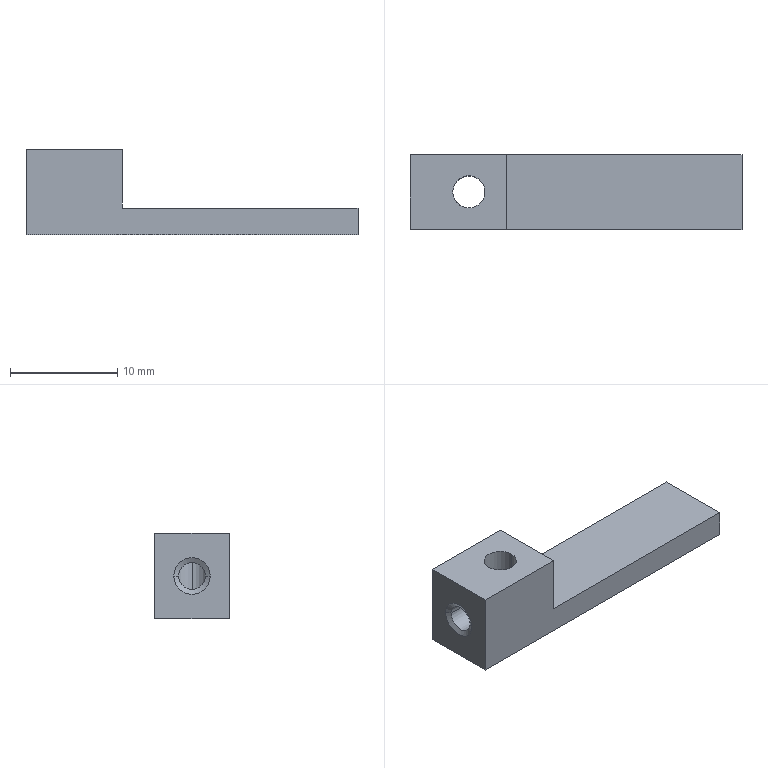Part | NX | 1 solid | 14 faces | box 31 x 7 x 8 mm | volume 811.579 mm3 | plane 8 | cylinder 4 | cone 2 | commonest cylinder face diameters 2.5 x2 3 x2
STEP:
#1=CARTESIAN_POINT('',(-15.5,3.5,-4.));
#2=VERTEX_POINT('',#1);
#3=CARTESIAN_POINT('',(-15.5,-3.5,-4.));
#4=VERTEX_POINT('',#3);
#5=CARTESIAN_POINT('',(-15.5,0.,-4.));
#6=DIRECTION('',(0.,-1.,0.));
#7=VECTOR('',#6,1000.);
#8=LINE('',#5,#7);
#9=EDGE_CURVE('',#2,#4,#8,.T.);
#10=ORIENTED_EDGE('',*,*,#9,.F.);
#11=CARTESIAN_POINT('',(15.5,3.5,-4.));
#12=VERTEX_POINT('',#11);
#13=CARTESIAN_POINT('',(-15.5,3.5,-4.));
#14=DIRECTION('',(1.,0.,0.));
#15=VECTOR('',#14,1000.);
#16=LINE('',#13,#15);
#17=EDGE_CURVE('',#2,#12,#16,.T.);
#18=ORIENTED_EDGE('',*,*,#17,.T.);
#19=CARTESIAN_POINT('',(15.5,-3.5,-4.));
#20=VERTEX_POINT('',#19);
#21=CARTESIAN_POINT('',(15.5,3.5,-4.));
#22=DIRECTION('',(0.,-1.,0.));
#23=VECTOR('',#22,1000.);
#24=LINE('',#21,#23);
#25=EDGE_CURVE('',#12,#20,#24,.T.);
#26=ORIENTED_EDGE('',*,*,#25,.T.);
#27=CARTESIAN_POINT('',(15.5,-3.5,-4.));
#28=DIRECTION('',(-1.,0.,0.));
#29=VECTOR('',#28,1000.);
#30=LINE('',#27,#29);
#31=EDGE_CURVE('',#20,#4,#30,.T.);
#32=ORIENTED_EDGE('',*,*,#31,.T.);
#33=EDGE_LOOP('',(#10,#18,#26,#32));
#34=FACE_BOUND('',#33,.T.);
#35=CARTESIAN_POINT('',(-8.5,0.,-4.));
#36=VERTEX_POINT('',#35);
#37=CARTESIAN_POINT('',(-11.5,0.,-4.));
#38=VERTEX_POINT('',#37);
#39=CARTESIAN_POINT('',(-10.,0.,-4.));
#40=DIRECTION('',(0.,0.,1.));
#41=DIRECTION('',(1.,0.,0.));
#42=AXIS2_PLACEMENT_3D('',#39,#40,#41);
#43=CIRCLE('',#42,1.5);
#44=EDGE_CURVE('',#36,#38,#43,.T.);
#45=ORIENTED_EDGE('',*,*,#44,.T.);
#46=CARTESIAN_POINT('',(-10.,0.,-4.));
#47=DIRECTION('',(0.,0.,1.));
#48=DIRECTION('',(1.,0.,0.));
#49=AXIS2_PLACEMENT_3D('',#46,#47,#48);
#50=CIRCLE('',#49,1.5);
#51=EDGE_CURVE('',#38,#36,#50,.T.);
#52=ORIENTED_EDGE('',*,*,#51,.T.);
#53=EDGE_LOOP('',(#45,#52));
#54=FACE_BOUND('',#53,.T.);
#55=CARTESIAN_POINT('',(0.,0.,-4.));
#56=DIRECTION('',(0.,0.,1.));
#57=DIRECTION('',(1.,0.,0.));
#58=AXIS2_PLACEMENT_3D('',#55,#56,#57);
#59=PLANE('',#58);
#60=ADVANCED_FACE('',(#34,#54),#59,.F.);
#61=ORIENTED_EDGE('',*,*,#9,.T.);
#62=CARTESIAN_POINT('',(-15.5,-3.5,4.));
#63=VERTEX_POINT('',#62);
#64=CARTESIAN_POINT('',(-15.5,-3.5,0.));
#65=DIRECTION('',(0.,0.,-1.));
#66=VECTOR('',#65,1000.);
#67=LINE('',#64,#66);
#68=EDGE_CURVE('',#63,#4,#67,.T.);
#69=ORIENTED_EDGE('',*,*,#68,.F.);
#70=CARTESIAN_POINT('',(-15.5,3.5,4.));
#71=VERTEX_POINT('',#70);
#72=CARTESIAN_POINT('',(-15.5,0.,4.));
#73=DIRECTION('',(0.,-1.,0.));
#74=VECTOR('',#73,1000.);
#75=LINE('',#72,#74);
#76=EDGE_CURVE('',#71,#63,#75,.T.);
#77=ORIENTED_EDGE('',*,*,#76,.F.);
#78=CARTESIAN_POINT('',(-15.5,3.5,0.));
#79=DIRECTION('',(0.,0.,1.));
#80=VECTOR('',#79,1000.);
#81=LINE('',#78,#80);
#82=EDGE_CURVE('',#2,#71,#81,.T.);
#83=ORIENTED_EDGE('',*,*,#82,.F.);
#84=EDGE_LOOP('',(#61,#69,#77,#83));
#85=FACE_BOUND('',#84,.T.);
#86=CARTESIAN_POINT('',(-15.5,-1.7,0.));
#87=VERTEX_POINT('',#86);
#88=CARTESIAN_POINT('',(-15.5,1.7,0.));
#89=VERTEX_POINT('',#88);
#90=CARTESIAN_POINT('',(-15.5,0.,0.));
#91=DIRECTION('',(-1.,0.,0.));
#92=DIRECTION('',(0.,1.,0.));
#93=AXIS2_PLACEMENT_3D('',#90,#91,#92);
#94=CIRCLE('',#93,1.7);
#95=EDGE_CURVE('',#87,#89,#94,.T.);
#96=ORIENTED_EDGE('',*,*,#95,.F.);
#97=CARTESIAN_POINT('',(-15.5,0.,0.));
#98=DIRECTION('',(-1.,0.,0.));
#99=DIRECTION('',(0.,1.,0.));
#100=AXIS2_PLACEMENT_3D('',#97,#98,#99);
#101=CIRCLE('',#100,1.7);
#102=EDGE_CURVE('',#89,#87,#101,.T.);
#103=ORIENTED_EDGE('',*,*,#102,.F.);
#104=EDGE_LOOP('',(#96,#103));
#105=FACE_BOUND('',#104,.T.);
#106=CARTESIAN_POINT('',(-15.5,3.5,-4.));
#107=DIRECTION('',(-1.,0.,0.));
#108=DIRECTION('',(0.,0.,1.));
#109=AXIS2_PLACEMENT_3D('',#106,#107,#108);
#110=PLANE('',#109);
#111=ADVANCED_FACE('',(#85,#105),#110,.T.);
#112=CARTESIAN_POINT('',(-6.5,3.5,-1.5));
#113=VERTEX_POINT('',#112);
#114=CARTESIAN_POINT('',(15.5,3.5,-1.5));
#115=VERTEX_POINT('',#114);
#116=CARTESIAN_POINT('',(-6.5,3.5,-1.5));
#117=DIRECTION('',(1.,0.,0.));
#118=VECTOR('',#117,1000.);
#119=LINE('',#116,#118);
#120=EDGE_CURVE('',#113,#115,#119,.T.);
#121=ORIENTED_EDGE('',*,*,#120,.T.);
#122=CARTESIAN_POINT('',(15.5,3.5,-1.5));
#123=DIRECTION('',(0.,0.,-1.));
#124=VECTOR('',#123,1000.);
#125=LINE('',#122,#124);
#126=EDGE_CURVE('',#115,#12,#125,.T.);
#127=ORIENTED_EDGE('',*,*,#126,.T.);
#128=ORIENTED_EDGE('',*,*,#17,.F.);
#129=ORIENTED_EDGE('',*,*,#82,.T.);
#130=CARTESIAN_POINT('',(-6.5,3.5,4.));
#131=VERTEX_POINT('',#130);
#132=CARTESIAN_POINT('',(-15.5,3.5,4.));
#133=DIRECTION('',(1.,0.,0.));
#134=VECTOR('',#133,1000.);
#135=LINE('',#132,#134);
#136=EDGE_CURVE('',#71,#131,#135,.T.);
#137=ORIENTED_EDGE('',*,*,#136,.T.);
#138=CARTESIAN_POINT('',(-6.5,3.5,-1.5));
#139=DIRECTION('',(0.,0.,1.));
#140=VECTOR('',#139,1000.);
#141=LINE('',#138,#140);
#142=EDGE_CURVE('',#113,#131,#141,.T.);
#143=ORIENTED_EDGE('',*,*,#142,.F.);
#144=EDGE_LOOP('',(#121,#127,#128,#129,#137,#143));
#145=FACE_BOUND('',#144,.T.);
#146=CARTESIAN_POINT('',(15.5,3.5,-4.));
#147=DIRECTION('',(0.,1.,0.));
#148=DIRECTION('',(1.,0.,0.));
#149=AXIS2_PLACEMENT_3D('',#146,#147,#148);
#150=PLANE('',#149);
#151=ADVANCED_FACE('',(#145),#150,.T.);
#152=CARTESIAN_POINT('',(-6.5,-3.5,-1.5));
#153=VERTEX_POINT('',#152);
#154=CARTESIAN_POINT('',(15.5,-3.5,-1.5));
#155=VERTEX_POINT('',#154);
#156=CARTESIAN_POINT('',(-6.5,-3.5,-1.5));
#157=DIRECTION('',(1.,0.,0.));
#158=VECTOR('',#157,1000.);
#159=LINE('',#156,#158);
#160=EDGE_CURVE('',#153,#155,#159,.T.);
#161=ORIENTED_EDGE('',*,*,#160,.T.);
#162=CARTESIAN_POINT('',(15.5,3.5,-1.5));
#163=DIRECTION('',(0.,-1.,0.));
#164=VECTOR('',#163,1000.);
#165=LINE('',#162,#164);
#166=EDGE_CURVE('',#115,#155,#165,.T.);
#167=ORIENTED_EDGE('',*,*,#166,.F.);
#168=ORIENTED_EDGE('',*,*,#120,.F.);
#169=CARTESIAN_POINT('',(-6.5,-3.5,-1.5));
#170=DIRECTION('',(0.,1.,0.));
#171=VECTOR('',#170,1000.);
#172=LINE('',#169,#171);
#173=EDGE_CURVE('',#153,#113,#172,.T.);
#174=ORIENTED_EDGE('',*,*,#173,.F.);
#175=EDGE_LOOP('',(#161,#167,#168,#174));
#176=FACE_BOUND('',#175,.T.);
#177=CARTESIAN_POINT('',(15.5,3.5,-1.5));
#178=DIRECTION('',(0.,0.,-1.));
#179=DIRECTION('',(0.,-1.,0.));
#180=AXIS2_PLACEMENT_3D('',#177,#178,#179);
#181=PLANE('',#180);
#182=ADVANCED_FACE('',(#176),#181,.F.);
#183=ORIENTED_EDGE('',*,*,#160,.F.);
#184=CARTESIAN_POINT('',(-6.5,-3.5,4.));
#185=VERTEX_POINT('',#184);
#186=CARTESIAN_POINT('',(-6.5,-3.5,-1.5));
#187=DIRECTION('',(0.,0.,1.));
#188=VECTOR('',#187,1000.);
#189=LINE('',#186,#188);
#190=EDGE_CURVE('',#153,#185,#189,.T.);
#191=ORIENTED_EDGE('',*,*,#190,.T.);
#192=CARTESIAN_POINT('',(-6.5,-3.5,4.));
#193=DIRECTION('',(-1.,0.,0.));
#194=VECTOR('',#193,1000.);
#195=LINE('',#192,#194);
#196=EDGE_CURVE('',#185,#63,#195,.T.);
#197=ORIENTED_EDGE('',*,*,#196,.T.);
#198=ORIENTED_EDGE('',*,*,#68,.T.);
#199=ORIENTED_EDGE('',*,*,#31,.F.);
#200=CARTESIAN_POINT('',(15.5,-3.5,-1.5));
#201=DIRECTION('',(0.,0.,-1.));
#202=VECTOR('',#201,1000.);
#203=LINE('',#200,#202);
#204=EDGE_CURVE('',#155,#20,#203,.T.);
#205=ORIENTED_EDGE('',*,*,#204,.F.);
#206=EDGE_LOOP('',(#183,#191,#197,#198,#199,#205));
#207=FACE_BOUND('',#206,.T.);
#208=CARTESIAN_POINT('',(-15.5,-3.5,-4.));
#209=DIRECTION('',(0.,-1.,0.));
#210=DIRECTION('',(0.,0.,-1.));
#211=AXIS2_PLACEMENT_3D('',#208,#209,#210);
#212=PLANE('',#211);
#213=ADVANCED_FACE('',(#207),#212,.T.);
#214=ORIENTED_EDGE('',*,*,#166,.T.);
#215=ORIENTED_EDGE('',*,*,#204,.T.);
#216=ORIENTED_EDGE('',*,*,#25,.F.);
#217=ORIENTED_EDGE('',*,*,#126,.F.);
#218=EDGE_LOOP('',(#214,#215,#216,#217));
#219=FACE_BOUND('',#218,.T.);
#220=CARTESIAN_POINT('',(15.5,-3.5,-4.));
#221=DIRECTION('',(1.,0.,0.));
#222=DIRECTION('',(0.,1.,0.));
#223=AXIS2_PLACEMENT_3D('',#220,#221,#222);
#224=PLANE('',#223);
#225=ADVANCED_FACE('',(#219),#224,.T.);
#226=CARTESIAN_POINT('',(-6.5,3.5,4.));
#227=DIRECTION('',(0.,-1.,0.));
#228=VECTOR('',#227,1000.);
#229=LINE('',#226,#228);
#230=EDGE_CURVE('',#131,#185,#229,.T.);
#231=ORIENTED_EDGE('',*,*,#230,.F.);
#232=ORIENTED_EDGE('',*,*,#136,.F.);
#233=ORIENTED_EDGE('',*,*,#76,.T.);
#234=ORIENTED_EDGE('',*,*,#196,.F.);
#235=EDGE_LOOP('',(#231,#232,#233,#234));
#236=FACE_BOUND('',#235,.T.);
#237=CARTESIAN_POINT('',(-11.5,0.,4.));
#238=VERTEX_POINT('',#237);
#239=CARTESIAN_POINT('',(-8.5,0.,4.));
#240=VERTEX_POINT('',#239);
#241=CARTESIAN_POINT('',(-10.,0.,4.));
#242=DIRECTION('',(0.,0.,1.));
#243=DIRECTION('',(1.,0.,0.));
#244=AXIS2_PLACEMENT_3D('',#241,#242,#243);
#245=CIRCLE('',#244,1.5);
#246=EDGE_CURVE('',#238,#240,#245,.T.);
#247=ORIENTED_EDGE('',*,*,#246,.F.);
#248=CARTESIAN_POINT('',(-10.,0.,4.));
#249=DIRECTION('',(0.,0.,1.));
#250=DIRECTION('',(1.,0.,0.));
#251=AXIS2_PLACEMENT_3D('',#248,#249,#250);
#252=CIRCLE('',#251,1.5);
#253=EDGE_CURVE('',#240,#238,#252,.T.);
#254=ORIENTED_EDGE('',*,*,#253,.F.);
#255=EDGE_LOOP('',(#247,#254));
#256=FACE_BOUND('',#255,.T.);
#257=CARTESIAN_POINT('',(0.,0.,4.));
#258=DIRECTION('',(0.,0.,1.));
#259=DIRECTION('',(1.,0.,0.));
#260=AXIS2_PLACEMENT_3D('',#257,#258,#259);
#261=PLANE('',#260);
#262=ADVANCED_FACE('',(#236,#256),#261,.T.);
#263=ORIENTED_EDGE('',*,*,#230,.T.);
#264=ORIENTED_EDGE('',*,*,#190,.F.);
#265=ORIENTED_EDGE('',*,*,#173,.T.);
#266=ORIENTED_EDGE('',*,*,#142,.T.);
#267=EDGE_LOOP('',(#263,#264,#265,#266));
#268=FACE_BOUND('',#267,.T.);
#269=CARTESIAN_POINT('',(-6.5,3.5,-1.5));
#270=DIRECTION('',(-1.,0.,0.));
#271=DIRECTION('',(0.,0.,1.));
#272=AXIS2_PLACEMENT_3D('',#269,#270,#271);
#273=PLANE('',#272);
#274=ADVANCED_FACE('',(#268),#273,.F.);
#275=ORIENTED_EDGE('',*,*,#44,.F.);
#276=CARTESIAN_POINT('',(-8.5,0.,-4.));
#277=DIRECTION('',(0.,0.,1.));
#278=VECTOR('',#277,1000.);
#279=LINE('',#276,#278);
#280=EDGE_CURVE('',#36,#240,#279,.T.);
#281=ORIENTED_EDGE('',*,*,#280,.T.);
#282=ORIENTED_EDGE('',*,*,#253,.T.);
#283=CARTESIAN_POINT('',(-11.5,0.,1.25));
#284=VERTEX_POINT('',#283);
#285=CARTESIAN_POINT('',(-11.5,0.,-4.));
#286=DIRECTION('',(0.,0.,1.));
#287=VECTOR('',#286,1000.);
#288=LINE('',#285,#287);
#289=EDGE_CURVE('',#284,#238,#288,.T.);
#290=ORIENTED_EDGE('',*,*,#289,.F.);
#291=CARTESIAN_POINT('',(-10.829,1.25,0.));
#292=VERTEX_POINT('',#291);
#293=CARTESIAN_POINT('',(-11.5,0.,1.25));
#294=CARTESIAN_POINT('',(-11.5,0.342,1.25));
#295=CARTESIAN_POINT('',(-11.245,0.9913,0.9644));
#296=CARTESIAN_POINT('',(-10.83,1.25,0.3175));
#297=CARTESIAN_POINT('',(-10.829,1.25,0.));
#298=B_SPLINE_CURVE_WITH_KNOTS('',3,(#293,#294,#295,#296,#297),.UNSPECIFIED.,.F.,.F.,(4,1,4),(0.,0.5,1.),.UNSPECIFIED.);
#299=EDGE_CURVE('',#284,#292,#298,.T.);
#300=ORIENTED_EDGE('',*,*,#299,.T.);
#301=CARTESIAN_POINT('',(-11.5,0.,-1.25));
#302=VERTEX_POINT('',#301);
#303=CARTESIAN_POINT('',(-10.829,1.25,0.));
#304=CARTESIAN_POINT('',(-10.83,1.25,-0.3173));
#305=CARTESIAN_POINT('',(-11.245,0.9912,-0.9645));
#306=CARTESIAN_POINT('',(-11.5,0.3421,-1.25));
#307=CARTESIAN_POINT('',(-11.5,0.,-1.25));
#308=B_SPLINE_CURVE_WITH_KNOTS('',3,(#303,#304,#305,#306,#307),.UNSPECIFIED.,.F.,.F.,(4,1,4),(0.,0.5,1.),.UNSPECIFIED.);
#309=EDGE_CURVE('',#292,#302,#308,.T.);
#310=ORIENTED_EDGE('',*,*,#309,.T.);
#311=CARTESIAN_POINT('',(-11.5,0.,-4.));
#312=DIRECTION('',(0.,0.,1.));
#313=VECTOR('',#312,1000.);
#314=LINE('',#311,#313);
#315=EDGE_CURVE('',#38,#302,#314,.T.);
#316=ORIENTED_EDGE('',*,*,#315,.F.);
#317=EDGE_LOOP('',(#275,#281,#282,#290,#300,#310,#316));
#318=FACE_BOUND('',#317,.T.);
#319=CARTESIAN_POINT('',(-10.,0.,-4.));
#320=DIRECTION('',(0.,0.,1.));
#321=DIRECTION('',(1.,0.,0.));
#322=AXIS2_PLACEMENT_3D('',#319,#320,#321);
#323=CYLINDRICAL_SURFACE('',#322,1.5);
#324=ADVANCED_FACE('',(#318),#323,.F.);
#325=ORIENTED_EDGE('',*,*,#309,.F.);
#326=CARTESIAN_POINT('',(-15.24,1.25,0.));
#327=VERTEX_POINT('',#326);
#328=CARTESIAN_POINT('',(-15.5,1.25,0.));
#329=DIRECTION('',(-1.,0.,0.));
#330=VECTOR('',#329,1000.);
#331=LINE('',#328,#330);
#332=EDGE_CURVE('',#292,#327,#331,.T.);
#333=ORIENTED_EDGE('',*,*,#332,.T.);
#334=CARTESIAN_POINT('',(-15.24,-1.25,0.));
#335=VERTEX_POINT('',#334);
#336=CARTESIAN_POINT('',(-15.24,0.,0.));
#337=DIRECTION('',(-1.,0.,0.));
#338=DIRECTION('',(0.,1.,0.));
#339=AXIS2_PLACEMENT_3D('',#336,#337,#338);
#340=CIRCLE('',#339,1.25);
#341=EDGE_CURVE('',#327,#335,#340,.T.);
#342=ORIENTED_EDGE('',*,*,#341,.T.);
#343=CARTESIAN_POINT('',(-10.829,-1.25,0.));
#344=VERTEX_POINT('',#343);
#345=CARTESIAN_POINT('',(-15.5,-1.25,0.));
#346=DIRECTION('',(-1.,0.,0.));
#347=VECTOR('',#346,1000.);
#348=LINE('',#345,#347);
#349=EDGE_CURVE('',#344,#335,#348,.T.);
#350=ORIENTED_EDGE('',*,*,#349,.F.);
#351=CARTESIAN_POINT('',(-10.829,-1.25,0.));
#352=CARTESIAN_POINT('',(-10.829,-1.25,-0.1449));
#353=CARTESIAN_POINT('',(-10.935,-1.174,-0.4572));
#354=CARTESIAN_POINT('',(-11.039,-1.09,-0.6325));
#355=CARTESIAN_POINT('',(-11.182,-0.9256,-0.8438));
#356=CARTESIAN_POINT('',(-11.202,-0.8996,-0.8699));
#357=CARTESIAN_POINT('',(-11.345,-0.6794,-1.063));
#358=CARTESIAN_POINT('',(-11.438,-0.4603,-1.174));
#359=CARTESIAN_POINT('',(-11.5,-0.1667,-1.25));
#360=CARTESIAN_POINT('',(-11.5,0.,-1.25));
#361=B_SPLINE_CURVE_WITH_KNOTS('',3,(#351,#352,#353,#354,#355,#356,#357,#358,#359,#360),.UNSPECIFIED.,.F.,.F.,(4,1,1,1,1,1,1,4),(0.,0.25,0.375,0.4375,0.5,0.625,0.75,1.),.UNSPECIFIED.);
#362=EDGE_CURVE('',#302,#344,#361,.F.);
#363=ORIENTED_EDGE('',*,*,#362,.F.);
#364=EDGE_LOOP('',(#325,#333,#342,#350,#363));
#365=FACE_BOUND('',#364,.T.);
#366=CARTESIAN_POINT('',(-15.5,0.,0.));
#367=DIRECTION('',(-1.,0.,0.));
#368=DIRECTION('',(0.,1.,0.));
#369=AXIS2_PLACEMENT_3D('',#366,#367,#368);
#370=CYLINDRICAL_SURFACE('',#369,1.25);
#371=ADVANCED_FACE('',(#365),#370,.F.);
#372=CARTESIAN_POINT('',(-15.24,0.,0.));
#373=DIRECTION('',(-1.,0.,0.));
#374=DIRECTION('',(0.,1.,0.));
#375=AXIS2_PLACEMENT_3D('',#372,#373,#374);
#376=CIRCLE('',#375,1.25);
#377=EDGE_CURVE('',#335,#327,#376,.T.);
#378=ORIENTED_EDGE('',*,*,#377,.F.);
#379=CARTESIAN_POINT('',(-15.24,-1.25,0.));
#380=DIRECTION('',(-0.5,-0.866,0.));
#381=VECTOR('',#380,1000.);
#382=LINE('',#379,#381);
#383=EDGE_CURVE('',#335,#87,#382,.T.);
#384=ORIENTED_EDGE('',*,*,#383,.T.);
#385=ORIENTED_EDGE('',*,*,#95,.T.);
#386=CARTESIAN_POINT('',(-15.24,1.25,0.));
#387=DIRECTION('',(-0.5,0.866,0.));
#388=VECTOR('',#387,1000.);
#389=LINE('',#386,#388);
#390=EDGE_CURVE('',#327,#89,#389,.T.);
#391=ORIENTED_EDGE('',*,*,#390,.F.);
#392=EDGE_LOOP('',(#378,#384,#385,#391));
#393=FACE_BOUND('',#392,.T.);
#394=CARTESIAN_POINT('',(-15.24,0.,0.));
#395=DIRECTION('',(-1.,0.,0.));
#396=DIRECTION('',(0.,1.,0.));
#397=AXIS2_PLACEMENT_3D('',#394,#395,#396);
#398=CONICAL_SURFACE('',#397,1.25,1.047);
#399=ADVANCED_FACE('',(#393),#398,.F.);
#400=ORIENTED_EDGE('',*,*,#390,.T.);
#401=ORIENTED_EDGE('',*,*,#102,.T.);
#402=ORIENTED_EDGE('',*,*,#383,.F.);
#403=ORIENTED_EDGE('',*,*,#341,.F.);
#404=EDGE_LOOP('',(#400,#401,#402,#403));
#405=FACE_BOUND('',#404,.T.);
#406=CARTESIAN_POINT('',(-15.24,0.,0.));
#407=DIRECTION('',(-1.,0.,0.));
#408=DIRECTION('',(0.,1.,0.));
#409=AXIS2_PLACEMENT_3D('',#406,#407,#408);
#410=CONICAL_SURFACE('',#409,1.25,1.047);
#411=ADVANCED_FACE('',(#405),#410,.F.);
#412=ORIENTED_EDGE('',*,*,#377,.T.);
#413=ORIENTED_EDGE('',*,*,#332,.F.);
#414=ORIENTED_EDGE('',*,*,#299,.F.);
#415=CARTESIAN_POINT('',(-11.5,0.,1.25));
#416=CARTESIAN_POINT('',(-11.5,-0.1667,1.25));
#417=CARTESIAN_POINT('',(-11.438,-0.4604,1.174));
#418=CARTESIAN_POINT('',(-11.345,-0.6792,1.063));
#419=CARTESIAN_POINT('',(-11.202,-0.8998,0.8698));
#420=CARTESIAN_POINT('',(-11.182,-0.9253,0.8441));
#421=CARTESIAN_POINT('',(-11.039,-1.09,0.6325));
#422=CARTESIAN_POINT('',(-10.935,-1.173,0.4548));
#423=CARTESIAN_POINT('',(-10.829,-1.25,0.1559));
#424=CARTESIAN_POINT('',(-10.829,-1.25,0.));
#425=B_SPLINE_CURVE_WITH_KNOTS('',3,(#415,#416,#417,#418,#419,#420,#421,#422,#423,#424),.UNSPECIFIED.,.F.,.F.,(4,1,1,1,1,1,1,4),(0.,0.25,0.375,0.5,0.5625,0.625,0.75,1.),.UNSPECIFIED.);
#426=EDGE_CURVE('',#344,#284,#425,.F.);
#427=ORIENTED_EDGE('',*,*,#426,.F.);
#428=ORIENTED_EDGE('',*,*,#349,.T.);
#429=EDGE_LOOP('',(#412,#413,#414,#427,#428));
#430=FACE_BOUND('',#429,.T.);
#431=CARTESIAN_POINT('',(-15.5,0.,0.));
#432=DIRECTION('',(-1.,0.,0.));
#433=DIRECTION('',(0.,1.,0.));
#434=AXIS2_PLACEMENT_3D('',#431,#432,#433);
#435=CYLINDRICAL_SURFACE('',#434,1.25);
#436=ADVANCED_FACE('',(#430),#435,.F.);
#437=ORIENTED_EDGE('',*,*,#246,.T.);
#438=ORIENTED_EDGE('',*,*,#280,.F.);
#439=ORIENTED_EDGE('',*,*,#51,.F.);
#440=ORIENTED_EDGE('',*,*,#315,.T.);
#441=ORIENTED_EDGE('',*,*,#362,.T.);
#442=ORIENTED_EDGE('',*,*,#426,.T.);
#443=ORIENTED_EDGE('',*,*,#289,.T.);
#444=EDGE_LOOP('',(#437,#438,#439,#440,#441,#442,#443));
#445=FACE_BOUND('',#444,.T.);
#446=CARTESIAN_POINT('',(-10.,0.,-4.));
#447=DIRECTION('',(0.,0.,1.));
#448=DIRECTION('',(1.,0.,0.));
#449=AXIS2_PLACEMENT_3D('',#446,#447,#448);
#450=CYLINDRICAL_SURFACE('',#449,1.5);
#451=ADVANCED_FACE('',(#445),#450,.F.);
#452=CLOSED_SHELL('',(#60,#111,#151,#182,#213,#225,#262,#274,#324,#371,#399,#411,#436,#451));
#453=MANIFOLD_SOLID_BREP('',#452);
#454=(LENGTH_UNIT()NAMED_UNIT(*)SI_UNIT(.MILLI.,.METRE.));
#455=UNCERTAINTY_MEASURE_WITH_UNIT(LENGTH_MEASURE(0.0508),#454,'','');
#456=(NAMED_UNIT(*)PLANE_ANGLE_UNIT()SI_UNIT($,.RADIAN.));
#457=(NAMED_UNIT(*)SI_UNIT($,.STERADIAN.)SOLID_ANGLE_UNIT());
#458=(GEOMETRIC_REPRESENTATION_CONTEXT(3)GLOBAL_UNCERTAINTY_ASSIGNED_CONTEXT((#455))GLOBAL_UNIT_ASSIGNED_CONTEXT((#454,#456,#457))REPRESENTATION_CONTEXT('',''));
#459=ADVANCED_BREP_SHAPE_REPRESENTATION('',(#453),#458);